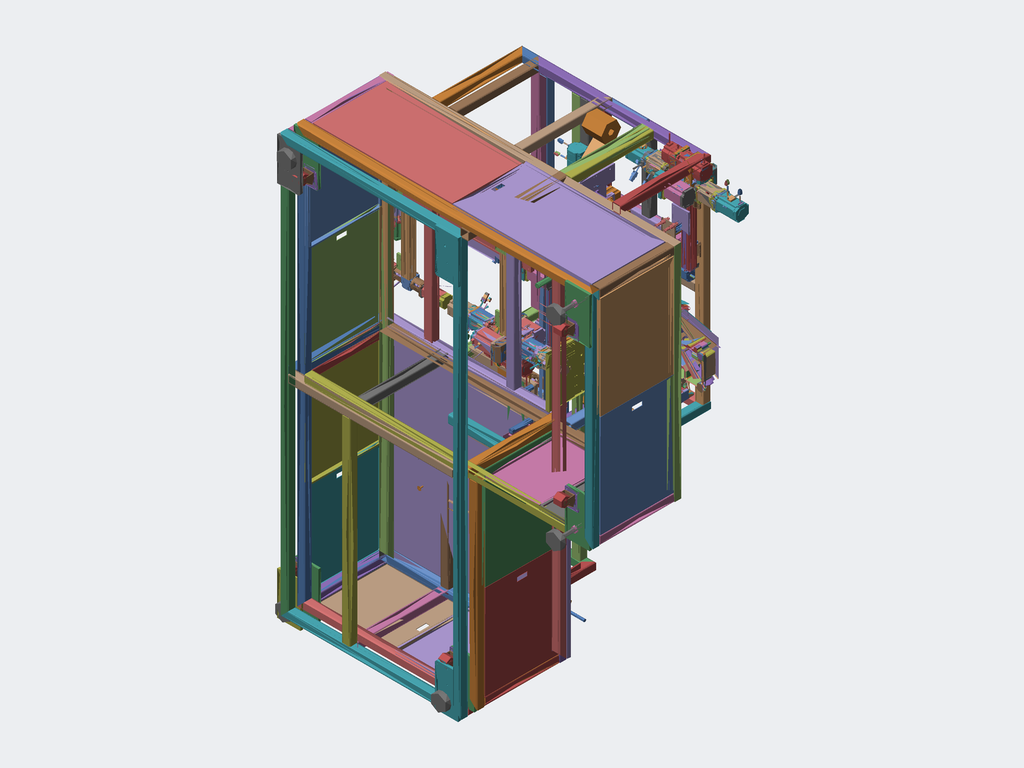Assembly | STEP file | 158 different items | 411 placed
Parts list (item | name | quantity | parent item | size | volume):
1 | - | x3 | in A14-05, A14-01 | 36 x 400 x 36 mm | 199320 mm3
2 | - | x4 | in A14-05, A14-01 | 120 x 120 x 120 mm | 1235023 mm3
3 | - | x1 | in A14-01 | 1150 x 1215 x 2550 mm | 25178560 mm3
4 | A14-004 | x1 | in A14-01 | 1200 x 20 x 1100 mm | 26268429 mm3
5 | 0303 sewing machinemodel | x1 | in A14-04 | - | -
6 | A14-006 | x8 | in A14-04 | 25 x 180 x 25 mm | 86683 mm3
7 | A14-007 | x1 | in A14-04 | 280 x 15 x 560 mm | 1039428 mm3
8 | A14-008 | x1 | in A14-04 | 290 x 20 x 750 mm | 2491365 mm3
9 | A14-005 | x2 | in 10 | 120.042 x 109.776 x 9.287 mm | 29092 mm3
10 | A14-009 | x1 | in A14-01 | - | -
11 | A14-010 | x1 | in A14-02 | 450 x 370 x 20 mm | 1407992 mm3
12 | A14-011 | x1 | in A14-02 | 450 x 370 x 20 mm | 1435092 mm3
13 | LC86HS150(shaft 14 length 32)- | x2 | in A14-02 | 86 x 86 x 182 mm | 1005876 mm3
14 | PF90-14-73-98.4-M5-20-L1 | x2 | in A14-02 | 90 x 150.5 x 90 mm | 705091 mm3
15 | A14-014 | x4 | in A14-02 | 45 x 95 x 20 mm | 53108 mm3
16 | A14-012 | x2 | in A14-02 | 60 x 310 x 60 mm | 431396 mm3
17 | A14-013 | x2 | in A14-02 | 60 x 310 x 60 mm | 430941 mm3
18 | A14-015 | x4 | in A14-02 | 40 x 14 x 39.975 mm | 13564 mm3
19 | A14-016 | x4 | in A14-02 | 280 x 16 x 16 mm | 56297 mm3
20 | A14-039 | x1 | in A14-02 | 100 x 320 x 10 mm | 307434 mm3
21 | A14-040 | x1 | in A14-02 | 38 x 320 x 10 mm | 121232 mm3
22 | - | x2 | in A14-02, A14-03 | - | -
23 | A14-018 | x1 | in A14-03 | 300 x 15 x 50 mm | 221576 mm3
24 | A14-020 | x1 | in A14-03 | 50 x 15 x 185 mm | 94203 mm3
25 | A14-021 | x1 | in A14-03 | 50 x 15 x 185 mm | 94219 mm3
26 | A14-025 | x1 | in A14-03 | 330 x 15 x 50 mm | 229412 mm3
27 | A14-019 | x1 | in A14-03 | 230 x 44 x 13 mm | 129953 mm3
28 | A14-022 | x2 | in A14-03 | 35 x 15 x 170 mm | 81962 mm3
29 | A14-028 | x1 | in A14-03 | 12 x 44 x 230 mm | 118590 mm3
30 | LSD15BK-HN-N-A-M4 | x2 | in A14-03 | 66.3 x 19.5 x 34 mm | 30804 mm3
31 | LSD15RLX170-S25-N-D | x2 | in A14-03 | 170 x 12.5 x 15 mm | 26475 mm3
32 | A14-023 | x1 | in A14-03 | 230 x 24 x 20 mm | 108684 mm3
33 | A14-024 | x1 | in A14-03 | 299 x 12 x 65 mm | 229704 mm3
34 | A14-029 | x1 | in A14-03 | - | -
35 | A14-026 | x1 | in A14-03 | 80 x 25 x 20 mm | 29104 mm3
36 | A14-027 | x1 | in A14-03 | 30 x 23 x 20 mm | 7977 mm3
37 | A14-030-1 | x1 | in A14-03 | 20 x 200 x 400 mm | 1595460 mm3
38 | A14-032 | x4 | in A14-03 | 25 x 130 x 25 mm | 62139 mm3
39 | A14-053 | x1 | in A14-03 | 204.473 x 29.929 x 260 mm | 95693 mm3
40 | - | x1 | in A14-01 | 100 x 200.5 x 1212 mm | 80600 mm3
41 | Copy of 50-2016 profile^K50A-1H20-S(formula driven)-L300-motor left- | x3 | in K50A-1H20-S(formula driven)-L300-motor left-_0 output shaft | 50 x 425 x 52.45 mm | 861534 mm3
42 | Copy of 50N support base^K50A-1H20-S(formula driven)-L300-motor left- | x6 | in K50A-1H20-S(formula driven)-L300-motor left-_0 output shaft | 82 x 32 x 80 mm | 67767 mm3
43 | Copy of K50-4 wheel slider (type B)^K50A-1H20-S(formula driven)-L300-motor left- | x3 | in K50A-1H20-S(formula driven)-L300-motor left-_0 output shaft | 140 x 34.5 x 102 mm | 434143 mm3
44 | Copy of 50-sensor^K50A-1H20-S(formula driven)-L300-motor left- | x9 | in K50A-1H20-S(formula driven)-L300-motor left-_0 output shaft | - | -
45 | Copy of K50-004 sensing plate^K50A-1H20-S(formula driven)-L300-motor left- | x3 | in K50A-1H20-S(formula driven)-L300-motor left-_0 output shaft | 20 x 33 x 15 mm | 1039 mm3
46 | Copy of K50-001A^K50A-1H20-S(formula driven)-L300-motor left- | x6 | in K50A-1H20-S(formula driven)-L300-motor left-_0 output shaft | 50 x 65 x 67.5 mm | 172642 mm3
47 | Copy of K50-right output shaft^K50A-1H20-S(formula driven)-L300-motor left- | x6 | in K50A-1H20-S(formula driven)-L300-motor left-_0 output shaft | 75.1 x 65 x 67.5 mm | 175546 mm3
48 | Copy of K50-double output shaft^K50A-1H20-S(formula driven)-L300-motor left- | x6 | in K50A-1H20-S(formula driven)-L300-motor left-_0 output shaft | 100.2 x 65 x 67.5 mm | 178596 mm3
49 | Copy of K50-left output shaft^K50A-1H20-S(formula driven)-L300-motor left- | x6 | in K50A-1H20-S(formula driven)-L300-motor left-_0 output shaft | 75.1 x 65 x 67.5 mm | 175546 mm3
50 | Copy of CZ002-400W side link 2:1(K60)^K50A-1H20-S(formula driven)-L300-motor left- | x6 | in K50A-1H20-S(formula driven)-L300-motor left-_0 output shaft | 161.001 x 70 x 175.5 mm | 580294 mm3
51 | Copy of CZ006-400W side link 3:1(K60)^K50A-1H20-S(formula driven)-L300-motor left- | x6 | in K50A-1H20-S(formula driven)-L300-motor left-_0 output shaft | 88 x 199.001 x 175.5 mm | 672015 mm3
52 | Copy of C0045-60 side link 2:1(K60)^K50A-1H20-S(formula driven)-L300-motor left- | x6 | in K50A-1H20-S(formula driven)-L300-motor left-_0 output shaft | 136.5 x 70 x 107.5 mm | 331047 mm3
53 | Copy of 400W gearbox assembly (universal motor base plus Q15)^K50A-1H20-S(formula driven)-L300-motor left- | x6 | in K50A-1H20-S(formula driven)-L300-motor left-_0 output shaft | 131.976 x 164.111 x 242.5 mm | 719537 mm3
54 | Copy of 400W motor assembly (60 motor base)^K50A-1H20-S(formula driven)-L300-motor left- | x6 | in K50A-1H20-S(formula driven)-L300-motor left-_0 output shaft | 65 x 95.5 x 200.5 mm | 502014 mm3
55 | Copy of 400W motor assembly (universal motor base)^K50A-1H20-S(formula driven)-L300-motor left- | x6 | in K50A-1H20-S(formula driven)-L300-motor left-_0 output shaft | 88.621 x 88.621 x 198.5 mm | 512392 mm3
56 | Copy of 60 motor assembly (universal motor base)^K50A-1H20-S(formula driven)-L300-motor left- | x6 | in K50A-1H20-S(formula driven)-L300-motor left-_0 output shaft | 82.65 x 82.65 x 148.5 mm | 366455 mm3
57 | Copy of 57 motor assembly (universal motor base)^K50A-1H20-S(formula driven)-L300-motor left- | x6 | in K50A-1H20-S(formula driven)-L300-motor left-_0 output shaft | 82.368 x 82.368 x 117.5 mm | 245014 mm3
58 | Copy of CZ031-57 side link 2:1(60-60N)^K50A-1H20-S(formula driven)-L300-motor left- | x6 | in K50A-1H20-S(formula driven)-L300-motor left-_0 output shaft | 60 x 146.25 x 90.3 mm | 270957 mm3
59 | Copy of CZ033-57 side link 3:1(60-60N)^K50A-1H20-S(formula driven)-L300-motor left- | x6 | in K50A-1H20-S(formula driven)-L300-motor left-_0 output shaft | 60 x 146.5 x 90.3 mm | 285335 mm3
60 | Copy of 86 motor assembly (universal motor base)^K50A-1H20-S(formula driven)-L300-motor left- | x6 | in K50A-1H20-S(formula driven)-L300-motor left-_0 output shaft | 86.045 x 86.045 x 193 mm | 941997 mm3
61 | Copy of CZ020-86 side link 2:1(K60)^K50A-1H20-S(formula driven)-L300-motor left- | x6 | in K50A-1H20-S(formula driven)-L300-motor left-_0 output shaft | 88 x 164.5 x 162 mm | 999458 mm3
62 | Copy of 90 reducer-universal motor base^K50A-1H20-S(formula driven)-L300-motor left- | x6 | in K50A-1H20-S(formula driven)-L300-motor left-_0 output shaft | 176.65 x 90 x 314 mm | 1490817 mm3
63 | Copy of 100W motor assembly (universal motor base)^K50A-1H20-S(formula driven)-L300-motor left- | x6 | in K50A-1H20-S(formula driven)-L300-motor left-_0 output shaft | 82.368 x 82.368 x 154.9 mm | 253997 mm3
64 | Copy of 750W motor assembly (universal motor base)^K50A-1H20-S(formula driven)-L300-motor left- | x6 | in K50A-1H20-S(formula driven)-L300-motor left-_0 output shaft | 82.368 x 139.887 x 214.5 mm | 943398 mm3
65 | Copy of CZ013-750W side link 2:1(K60)^K50A-1H20-S(formula driven)-L300-motor left- | x6 | in K50A-1H20-S(formula driven)-L300-motor left-_0 output shaft | 88 x 238.88 x 185 mm | 1086886 mm3
66 | Copy of hard limit assembly (right)^K50A-1H20-S(formula driven)-L300-motor left- | x3 | in K50A-1H20-S(formula driven)-L300-motor left-_0 output shaft | 24 x 15.5 x 40 mm | 6072 mm3
67 | Copy of hard limit assembly (left)^K50A-1H20-S(formula driven)-L300-motor left- | x3 | in K50A-1H20-S(formula driven)-L300-motor left-_0 output shaft | 24 x 15.5 x 40 mm | 6072 mm3
68 | A14-033 | x4 | in A14-01 | 250 x 10 x 130 mm | 324205 mm3
69 | vacuum suction cup assembly 4.5-fold bellows type standard type GXSE[GXSE-d20-20] | x8 | in A14-06 | 23.018 x 98.5 x 21.189 mm | 17845 mm3
70 | A14-034 | x3 | in A14-06, A14-13 | 10 x 100 x 120 mm | 119050 mm3
71 | A14-038 | x2 | in A14-06 | 125 x 80 x 8 mm | 15817 mm3
72 | - | x7 | in A14-06, A14-12, A14-13 | 66.5 x 47 x 20 mm | 46742 mm3
73 | A14-004-1 | x1 | in A14-01 | - | -
74 | A14-051 | x4 | in A14-10 | 25 x 207 x 25 mm | 99936 mm3
75 | A14-050 | x1 | in A14-10 | 20 x 210 x 470 mm | 1969460 mm3
76 | 311 base plate shell | x1 | in A14-11 | - | -
77 | - | x1 | in A14-11 | 100 x 58 x 40 mm | 26779 mm3
78 | 311 square head shell^2210 housing punching machine(2)_2210 housing punching machine | x1 | in A14-11 | - | -
79 | A14-052 | x1 | in A14-11 | 520 x 2 x 240 mm | 145187 mm3
80 | - | x1 | in A14-11 | 112.05 x 65 x 2.65 mm | 17494 mm3
81 | A14-062 | x1 | in A14-11 | 153 x 225 x 1.5 mm | 17798 mm3
82 | Copy of K50-right output shaft^K50A-1H20-S(formula driven)-L1200 right | x2 | in K50A-1H20-S(formula driven)-L1200 right_0 output shaft | - | -
83 | Copy of 50-sensor^K50A-1H20-S(formula driven)-L1200 right | x6 | in K50A-1H20-S(formula driven)-L1200 right_0 output shaft | 48.5 x 21.5 x 13.5 mm | 3491 mm3
84 | Copy of 50-2016 profile^K50A-1H20-S(formula driven)-L1200 right | x2 | in K50A-1H20-S(formula driven)-L1200 right_0 output shaft | 50 x 565 x 52.45 mm | 1145333 mm3
85 | Copy of 50N support base^K50A-1H20-S(formula driven)-L1200 right | x4 | in K50A-1H20-S(formula driven)-L1200 right_0 output shaft | 82 x 32 x 80 mm | 67767 mm3
86 | Copy of K50-4 wheel slider (type B)^K50A-1H20-S(formula driven)-L1200 right | x2 | in K50A-1H20-S(formula driven)-L1200 right_0 output shaft | 140 x 34.5 x 102 mm | 434143 mm3
87 | Copy of K50-left output shaft^K50A-1H20-S(formula driven)-L1200 right | x2 | in K50A-1H20-S(formula driven)-L1200 right_0 output shaft | 75.1 x 65 x 67.5 mm | 175546 mm3
88 | Copy of CZ006-400W side link 3:1(K60)^K50A-1H20-S(formula driven)-L1200 right | x2 | in K50A-1H20-S(formula driven)-L1200 right_0 output shaft | 88 x 199.001 x 175.5 mm | 672015 mm3
89 | Copy of CZ002-400W side link 2:1(K60)^K50A-1H20-S(formula driven)-L1200 right | x2 | in K50A-1H20-S(formula driven)-L1200 right_0 output shaft | 161.001 x 70 x 175.5 mm | 580294 mm3
90 | Copy of K50-001A^K50A-1H20-S(formula driven)-L1200 right | x4 | in K50A-1H20-S(formula driven)-L1200 right_0 output shaft | 50 x 65 x 67.5 mm | 172642 mm3
91 | Copy of K50-double output shaft^K50A-1H20-S(formula driven)-L1200 right | x2 | in K50A-1H20-S(formula driven)-L1200 right_0 output shaft | 100.2 x 65 x 67.5 mm | 178596 mm3
92 | Copy of K50-004 sensing plate^K50A-1H20-S(formula driven)-L1200 right | x2 | in K50A-1H20-S(formula driven)-L1200 right_0 output shaft | 20 x 33 x 15 mm | 1039 mm3
93 | Copy of 60 motor assembly (universal motor base)^K50A-1H20-S(formula driven)-L1200 right | x2 | in K50A-1H20-S(formula driven)-L1200 right_0 output shaft | 82.65 x 82.65 x 148.5 mm | 366455 mm3
94 | Copy of C0045-60 side link 2:1(K60)^K50A-1H20-S(formula driven)-L1200 right | x2 | in K50A-1H20-S(formula driven)-L1200 right_0 output shaft | 136.5 x 70 x 107.5 mm | 331047 mm3
95 | Copy of 400W gearbox assembly (universal motor base plus Q15)^K50A-1H20-S(formula driven)-L1200 right | x2 | in K50A-1H20-S(formula driven)-L1200 right_0 output shaft | 131.976 x 164.111 x 242.5 mm | 720796 mm3
96 | Copy of 400W motor assembly (universal motor base)^K50A-1H20-S(formula driven)-L1200 right | x2 | in K50A-1H20-S(formula driven)-L1200 right_0 output shaft | 88.621 x 88.621 x 198.5 mm | 512392 mm3
97 | Copy of 86 motor assembly (universal motor base)^K50A-1H20-S(formula driven)-L1200 right | x2 | in K50A-1H20-S(formula driven)-L1200 right_0 output shaft | 86.045 x 86.045 x 193 mm | 941997 mm3
98 | Copy of CZ031-57 side link 2:1(60-60N)^K50A-1H20-S(formula driven)-L1200 right | x2 | in K50A-1H20-S(formula driven)-L1200 right_0 output shaft | 60 x 146.25 x 90.3 mm | 270957 mm3
99 | Copy of 400W motor assembly (60 motor base)^K50A-1H20-S(formula driven)-L1200 right | x4 | in K50A-1H20-S(formula driven)-L1200 right_0 output shaft | - | 565676 mm3
100 | Copy of CZ033-57 side link 3:1(60-60N)^K50A-1H20-S(formula driven)-L1200 right | x2 | in K50A-1H20-S(formula driven)-L1200 right_0 output shaft | 60 x 146.5 x 90.3 mm | 285335 mm3
101 | Copy of 57 motor assembly (universal motor base)^K50A-1H20-S(formula driven)-L1200 right | x2 | in K50A-1H20-S(formula driven)-L1200 right_0 output shaft | 82.368 x 82.368 x 117.5 mm | 245014 mm3
102 | Copy of 100W motor assembly (universal motor base)^K50A-1H20-S(formula driven)-L1200 right | x2 | in K50A-1H20-S(formula driven)-L1200 right_0 output shaft | 82.368 x 82.368 x 154.9 mm | 253997 mm3
103 | Copy of 750W motor assembly (universal motor base)^K50A-1H20-S(formula driven)-L1200 right | x2 | in K50A-1H20-S(formula driven)-L1200 right_0 output shaft | 82.368 x 139.887 x 214.5 mm | 943398 mm3
104 | Copy of CZ020-86 side link 2:1(K60)^K50A-1H20-S(formula driven)-L1200 right | x2 | in K50A-1H20-S(formula driven)-L1200 right_0 output shaft | 88 x 164.5 x 162 mm | 999458 mm3
105 | Copy of CZ013-750W side link 2:1(K60)^K50A-1H20-S(formula driven)-L1200 right | x2 | in K50A-1H20-S(formula driven)-L1200 right_0 output shaft | 88 x 238.88 x 185 mm | 1086886 mm3
106 | Copy of hard limit assembly (right)^K50A-1H20-S(formula driven)-L1200 right | x1 | in K50A-1H20-S(formula driven)-L1200 right_0 output shaft | 24 x 15.5 x 40 mm | 6072 mm3
107 | Copy of 90 reducer-universal motor base^K50A-1H20-S(formula driven)-L1200 right | x2 | in K50A-1H20-S(formula driven)-L1200 right_0 output shaft | 176.65 x 90 x 314 mm | 1490817 mm3
108 | Copy of hard limit assembly (left)^K50A-1H20-S(formula driven)-L1200 right | x1 | in K50A-1H20-S(formula driven)-L1200 right_0 output shaft | 24 x 15.5 x 40 mm | 6072 mm3
109 | Copy of 50N support base^K50A-1H20-S(formula driven)-L700-motor left- | x3 | in K50A-1H20-S(formula driven)-L700-motor left-_0 output shaft | 82 x 32 x 80 mm | 67767 mm3
110 | Copy of 50-2016 profile^K50A-1H20-S(formula driven)-L700-motor left- | x1 | in K50A-1H20-S(formula driven)-L700-motor left-_0 output shaft | 50 x 815 x 52.45 mm | 1652118 mm3
111 | Copy of K50-004 sensing plate^K50A-1H20-S(formula driven)-L700-motor left- | x1 | in K50A-1H20-S(formula driven)-L700-motor left-_0 output shaft | 20 x 33 x 15 mm | 1039 mm3
112 | Copy of 50-sensor^K50A-1H20-S(formula driven)-L700-motor left- | x3 | in K50A-1H20-S(formula driven)-L700-motor left-_0 output shaft | 48.5 x 21.5 x 13.5 mm | 3491 mm3
113 | Copy of K50-001A^K50A-1H20-S(formula driven)-L700-motor left- | x2 | in K50A-1H20-S(formula driven)-L700-motor left-_0 output shaft | 50 x 65 x 67.5 mm | 172642 mm3
114 | Copy of K50-4 wheel slider (type B)^K50A-1H20-S(formula driven)-L700-motor left- | x1 | in K50A-1H20-S(formula driven)-L700-motor left-_0 output shaft | 140 x 34.5 x 102 mm | 434143 mm3
115 | Copy of CZ006-400W side link 3:1(K60)^K50A-1H20-S(formula driven)-L700-motor left- | x2 | in K50A-1H20-S(formula driven)-L700-motor left-_0 output shaft | 88 x 199.001 x 175.5 mm | 672015 mm3
116 | Copy of K50-right output shaft^K50A-1H20-S(formula driven)-L700-motor left- | x2 | in K50A-1H20-S(formula driven)-L700-motor left-_0 output shaft | 75.1 x 65 x 67.5 mm | 175722 mm3
117 | Copy of K50-double output shaft^K50A-1H20-S(formula driven)-L700-motor left- | x2 | in K50A-1H20-S(formula driven)-L700-motor left-_0 output shaft | 100.2 x 65 x 67.5 mm | 178596 mm3
118 | Copy of K50-left output shaft^K50A-1H20-S(formula driven)-L700-motor left- | x2 | in K50A-1H20-S(formula driven)-L700-motor left-_0 output shaft | 75.1 x 65 x 67.5 mm | 175546 mm3
119 | Copy of 400W motor assembly (universal motor base)^K50A-1H20-S(formula driven)-L700-motor left- | x2 | in K50A-1H20-S(formula driven)-L700-motor left-_0 output shaft | 88.621 x 88.621 x 198.5 mm | 512392 mm3
120 | Copy of 400W gearbox assembly (universal motor base plus Q15)^K50A-1H20-S(formula driven)-L700-motor left- | x2 | in K50A-1H20-S(formula driven)-L700-motor left-_0 output shaft | 131.976 x 164.111 x 242.5 mm | 719537 mm3
121 | Copy of CZ002-400W side link 2:1(K60)^K50A-1H20-S(formula driven)-L700-motor left- | x2 | in K50A-1H20-S(formula driven)-L700-motor left-_0 output shaft | 161.001 x 70 x 175.5 mm | 580294 mm3
122 | Copy of C0045-60 side link 2:1(K60)^K50A-1H20-S(formula driven)-L700-motor left- | x2 | in K50A-1H20-S(formula driven)-L700-motor left-_0 output shaft | 136.5 x 70 x 107.5 mm | 328495 mm3
123 | Copy of 400W motor assembly (60 motor base)^K50A-1H20-S(formula driven)-L700-motor left- | x2 | in K50A-1H20-S(formula driven)-L700-motor left-_0 output shaft | 65 x 95.5 x 200.5 mm | 502014 mm3
124 | Copy of 86 motor assembly (universal motor base)^K50A-1H20-S(formula driven)-L700-motor left- | x2 | in K50A-1H20-S(formula driven)-L700-motor left-_0 output shaft | 86.045 x 86.045 x 193 mm | 941997 mm3
125 | Copy of 57 motor assembly (universal motor base)^K50A-1H20-S(formula driven)-L700-motor left- | x2 | in K50A-1H20-S(formula driven)-L700-motor left-_0 output shaft | 82.368 x 82.368 x 117.5 mm | 245014 mm3
126 | Copy of CZ020-86 side link 2:1(K60)^K50A-1H20-S(formula driven)-L700-motor left- | x2 | in K50A-1H20-S(formula driven)-L700-motor left-_0 output shaft | 88 x 164.5 x 162 mm | 999458 mm3
127 | Copy of CZ033-57 side link 3:1(60-60N)^K50A-1H20-S(formula driven)-L700-motor left- | x2 | in K50A-1H20-S(formula driven)-L700-motor left-_0 output shaft | 60 x 146.5 x 90.3 mm | 285335 mm3
128 | Copy of 100W motor assembly (universal motor base)^K50A-1H20-S(formula driven)-L700-motor left- | x2 | in K50A-1H20-S(formula driven)-L700-motor left-_0 output shaft | 82.368 x 82.368 x 154.9 mm | 253997 mm3
129 | Copy of 60 motor assembly (universal motor base)^K50A-1H20-S(formula driven)-L700-motor left- | x2 | in K50A-1H20-S(formula driven)-L700-motor left-_0 output shaft | 82.65 x 82.65 x 148.5 mm | 366455 mm3
130 | Copy of CZ031-57 side link 2:1(60-60N)^K50A-1H20-S(formula driven)-L700-motor left- | x2 | in K50A-1H20-S(formula driven)-L700-motor left-_0 output shaft | 60 x 146.25 x 90.3 mm | 270957 mm3
131 | Copy of 90 reducer-universal motor base^K50A-1H20-S(formula driven)-L700-motor left- | x2 | in K50A-1H20-S(formula driven)-L700-motor left-_0 output shaft | 176.65 x 90 x 314 mm | 1490817 mm3
132 | Copy of hard limit assembly (right)^K50A-1H20-S(formula driven)-L700-motor left- | x1 | in K50A-1H20-S(formula driven)-L700-motor left-_0 output shaft | - | -
133 | Copy of 750W motor assembly (universal motor base)^K50A-1H20-S(formula driven)-L700-motor left- | x2 | in K50A-1H20-S(formula driven)-L700-motor left-_0 output shaft | 82.368 x 139.887 x 214.5 mm | 943398 mm3
134 | Copy of CZ013-750W side link 2:1(K60)^K50A-1H20-S(formula driven)-L700-motor left- | x2 | in K50A-1H20-S(formula driven)-L700-motor left-_0 output shaft | 88 x 238.88 x 185 mm | 1086886 mm3
135 | Copy of hard limit assembly (left)^K50A-1H20-S(formula driven)-L700-motor left- | x1 | in K50A-1H20-S(formula driven)-L700-motor left-_0 output shaft | 24 x 15.5 x 40 mm | 6072 mm3
136 | A14-060 | x1 | in A14-01 | 20 x 140 x 800 mm | 2235460 mm3
137 | A14-054 | x1 | in A14-12 | 430 x 10 x 480 mm | 1374000 mm3
138 | A14-057 | x1 | in A14-12 | 225 x 47 x 112.237 mm | 46754 mm3
139 | A14-056 | x1 | in A14-12 | 225 x 45 x 112.237 mm | 46079 mm3
140 | - | x2 | in A14-12 | 220 x 66.1 x 30 mm | 246050 mm3
141 | A14-055 | x1 | in A14-12 | 100 x 10 x 180 mm | 180000 mm3
142 | A14-058 | x2 | in A14-12 | 159 x 1.5 x 70 mm | 6015 mm3
143 | - | x2 | in A14-12 | 51.5 x 47 x 20 mm | 36061 mm3
144 | A14-059 | x2 | in A14-12 | 128 x 32.237 x 30 mm | 10459 mm3
145 | A14-08-1 | x1 | in A14-01 | - | -
146 | A14-061 | x1 | in A14-13 | 1.5 x 140 x 230 mm | 44100 mm3
147 | A14-08-2 | x1 | in A14-01 | - | -
148 | - | x1 | in A14-01 | 2550 x 1100 x 1800 mm | 25123488 mm3
149 | A14-066 | x5 | in A14-01 | 280 x 15 x 150 mm | 623398 mm3
150 | CGL01-D63 | x5 | in A14-01 | 82 x 96 x 111.5 mm | 244829 mm3
151 | WAM05-D100-M16-L100 | x5 | in A14-01 | 100 x 207 x 100 mm | 345017 mm3
152 | A14-Product-1 | x1 | in A14-01 | 399.758 x 100 x 500.012 mm | 1680 mm3
153 | A14-Product-2 | x1 | in A14-01 | 0.02 x 100 x 225 mm | 450 mm3
154 | - | x1 | in A14-01 | - | -
155 | Mirror Velcro | x1 | in A14-01 | 542.128 x 100 x 143.128 mm | 120000 mm3
156 | - | x1 | in Assembly 1 | 88 x 1.5 x 100 mm | 13200 mm3
157 | A14-Product-3 | x1 | in Assembly 1 | 225 x 0.2 x 100 mm | 4500 mm3
158 | - | x1 | in Assembly 1 | 55 x 1.5 x 100 mm | 8250 mm3
Placements (level | parent | child | x y z in mm | rotation matrix by rows), first 214 of 428 lines:
1 | A14-01 | A14-05 | 7.395 -242.555 146.98 | 1 0 0 0 0.995 0.1 0 -0.1 0.995
2 | A14-05 | subassembly 2 | -1394.407 492.899 1398.325 | 0 -1 0 1 0 0 0 0 1
2 | A14-05 | subassembly 2 | -1394.407 76.452 1362.677 | 0 -1 0 1 0 0 0 0 1
2 | A14-05 | subassembly 3 | -1394.407 492.899 1398.325 | 0 1 0 -0.7725 0 -0.635 -0.635 0 0.7725
1 | A14-01 | subassembly 3 | -1387.011 -30.182 1495.176 | 0 1 0 -0.7102 0 0.704 0.704 0 0.7102
1 | A14-01 | subassembly 4 | -1394.407 -687.101 2958.325 | 1 0 0 0 1 0 0 0 1
1 | A14-01 | A14-004 | -1394.407 -62.102 2283.325 | 0 0 -1 0 1 0 1 0 -0
1 | A14-01 | A14-04 | 19.784 0.0 -75.0 | 1 0 0 0 1 0 0 0 1
2 | A14-04 | 0303 sewing machinemodel | -1383.772 332.899 2064.075 | 0 -1 0 0 0 1 -1 0 0
2 | A14-04 | A14-006 | -1336.272 47.898 1955.575 | 1 0 0 0 -1 0 0 0 -1
2 | A14-04 | A14-007 | -1556.272 137.899 2070.575 | 0 0 -1 0 1 0 1 0 -0
2 | A14-04 | A14-008 | -1481.272 152.899 2070.575 | 0 0 -1 0 1 0 1 0 -0
2 | A14-04 | A14-006 | -1486.272 47.898 1955.575 | 1 0 0 0 -1 0 0 0 -1
2 | A14-04 | A14-006 | -1636.272 47.898 1955.575 | 1 0 0 0 -1 0 0 0 -1
2 | A14-04 | A14-006 | -1786.272 47.898 1955.575 | 1 0 0 0 -1 0 0 0 -1
2 | A14-04 | A14-006 | -1786.272 47.898 2185.575 | 1 0 0 0 -1 0 0 0 -1
2 | A14-04 | A14-006 | -1636.272 47.898 2185.575 | 1 0 0 0 -1 0 0 0 -1
2 | A14-04 | A14-006 | -1486.272 47.898 2185.575 | 1 0 0 0 -1 0 0 0 -1
2 | A14-04 | A14-006 | -1336.272 47.898 2185.575 | 1 0 0 0 -1 0 0 0 -1
1 | A14-01 | A14-009 | -1389.54 57.396 1881.186 | 0 -1 0 0 0 1 -1 0 -0
2 | A14-009 | A14-005 | 7.985 4.838 116.002 | 1 0 0 0 1 0 0 0 1
2 | A14-009 | A14-005 | 8.245 4.842 131.605 | 0.9994 9e-06 -0.03332 -9e-06 -1 -0.000555 -0.03332 0.000555 -0.9994
1 | A14-01 | A14-009 | -1394.407 172.899 1793.075 | 0 0 1 0 1 0 -1 0 0
1 | A14-01 | A14-02 | -1174.407 128.588 2254.397 | 0 0 -1 0 1 0 1 0 -0
2 | A14-02 | A14-010 | -8.822 14.311 370.0 | 1 0 0 0 1 0 0 0 1
2 | A14-02 | A14-011 | -8.822 14.311 70.0 | -1 0 0 0 1 0 0 0 -1
2 | A14-02 | LC86HS150(shaft 14 length 32)- | 34.178 -41.689 500.5 | 0 -1 0 -1 0 0 0 0 -1
2 | A14-02 | PF90-14-73-98.4-M5-20-L1 | -8.822 -84.689 380.0 | 1 0 0 0 0 1 0 -1 0
2 | A14-02 | A14-014 | -8.822 105.241 370.0 | 1 0 0 0 1 0 0 0 1
2 | A14-02 | A14-014 | -8.822 105.241 70.0 | -1 0 0 0 1 0 0 0 -1
2 | A14-02 | A14-012 | -8.822 77.741 375.0 | -0.8835 0 0.4684 -0.4684 0 -0.8835 0 -1 0
2 | A14-02 | A14-013 | -8.822 15.311 375.0 | 0.8247 0 -0.5656 0.5656 0 0.8247 0 -1 0
2 | A14-02 | A14-015 | 50.067 4.311 282.233 | 0.9619 0 0.2736 0.2736 0 -0.9619 0 1 -0
2 | A14-02 | A14-016 | 50.067 4.311 220.0 | 0 0 -1 0 1 0 1 0 0
2 | A14-02 | A14-016 | 50.067 -160.689 220.0 | 0 0 -1 0 1 0 1 0 0
2 | A14-02 | A14-016 | 282.289 -160.689 220.0 | 0 0 -1 0 1 0 1 0 0
2 | A14-02 | A14-016 | 282.289 4.311 220.0 | 0 0 -1 0 1 0 1 0 0
2 | A14-02 | A14-015 | 50.067 4.311 154.331 | 0.9911 0 -0.1331 -0.1331 0 -0.9911 0 1 -0
2 | A14-02 | A14-015 | 282.289 4.311 282.233 | 1 0 0 0 0 -1 0 1 -0
2 | A14-02 | A14-015 | 282.289 4.311 154.331 | 1 0 0 0 0 -1 0 1 -0
2 | A14-02 | A14-014 | 341.178 129.561 70.0 | -1 0 0 0 1 0 0 0 -1
2 | A14-02 | A14-014 | 341.178 129.561 370.0 | 1 0 0 0 1 0 0 0 1
2 | A14-02 | A14-012 | 341.178 102.061 375.0 | -0.9187 0 0.3949 -0.3949 0 -0.9187 0 -1 0
2 | A14-02 | A14-013 | 341.178 15.311 375.0 | 0.8247 0 -0.5656 0.5656 0 0.8247 0 -1 0
2 | A14-02 | PF90-14-73-98.4-M5-20-L1 | 341.178 -84.689 380.0 | 1 0 0 0 0 1 0 -1 0
2 | A14-02 | LC86HS150(shaft 14 length 32)- | 384.178 -41.689 500.5 | 0 -1 0 -1 0 0 0 0 -1
2 | A14-02 | A14-039 | 341.178 204.311 220.0 | -1 0 0 0 0 1 0 1 -0
2 | A14-02 | A14-040 | 341.178 182.061 220.0 | -1 0 0 0 0 1 0 1 -0
2 | A14-02 | subassembly 5 | 341.178 209.311 220.0 | 0 -1 0 1 0 0 0 0 1
1 | A14-01 | A14-03 | -1341.395 81.548 2180.575 | 1 0 0 0 1 0 0 0 1
2 | A14-03 | A14-018 | -53.012 33.851 520.0 | 1 0 0 0 1 0 0 0 1
2 | A14-03 | A14-020 | -203.012 118.851 520.0 | 0 -1 0 0 0 -1 1 0 0
2 | A14-03 | A14-021 | 96.988 118.851 520.0 | 0 1 0 0 0 -1 -1 0 0
2 | A14-03 | A14-025 | -53.012 211.351 520.0 | 1 0 0 0 1 0 0 0 1
2 | A14-03 | A14-019 | -53.012 63.351 538.5 | -1 0 0 0 -1 0 0 0 1
2 | A14-03 | A14-022 | 79.488 126.351 545.0 | -1 0 0 0 0 -1 0 -1 0
2 | A14-03 | A14-022 | -185.512 126.351 545.0 | -1 0 0 0 0 -1 0 -1 0
2 | A14-03 | A14-028 | -53.012 63.351 526.0 | 0 0 1 0 1 0 -1 0 -0
2 | A14-03 | LSD15BK-HN-N-A-M4 | -185.512 139.601 508.0 | 0 0 -1 1 0 0 0 -1 0
2 | A14-03 | LSD15RLX170-S25-N-D | -185.512 41.351 532.0 | 0 0 -1 1 0 0 0 -1 0
2 | A14-03 | LSD15RLX170-S25-N-D | 79.488 41.351 532.0 | 0 0 -1 1 0 0 0 -1 0
2 | A14-03 | LSD15BK-HN-N-A-M4 | 79.488 139.601 508.0 | 0 0 -1 1 0 0 0 -1 0
2 | A14-03 | A14-023 | -53.012 162.101 520.0 | 1 0 0 0 0 1 0 -1 -0
2 | A14-03 | A14-024 | -53.012 139.601 502.0 | -1 0 0 0 0 -1 0 -1 0
2 | A14-03 | A14-029 | -53.012 110.601 513.0 | 0 0 1 0 1 0 -1 0 0
2 | A14-03 | subassembly 5 | -53.012 226.351 520.0 | 0 -1 0 1 0 0 0 0 1
2 | A14-03 | A14-026 | -53.012 172.101 520.0 | 1 0 0 0 1 0 0 0 1
2 | A14-03 | A14-027 | -53.012 181.101 520.0 | 1 0 0 0 1 0 0 0 1
2 | A14-03 | A14-030-1 | -53.012 16.351 595.0 | 0 0 -1 -1 0 0 0 1 0
2 | A14-03 | A14-032 | -238.012 -58.649 680.0 | 1 0 0 0 1 0 0 0 1
2 | A14-03 | A14-032 | 131.988 -58.649 680.0 | 1 0 0 0 1 0 0 0 1
2 | A14-03 | A14-032 | 131.988 -58.649 510.0 | 1 0 0 0 1 0 0 0 1
2 | A14-03 | A14-032 | -238.012 -58.649 510.0 | -0.8428 0 -0.5383 0 1 0 0.5383 0 -0.8428
2 | A14-03 | A14-053 | -53.012 55.422 545.0 | -1 0 0 0 1 0 0 0 -1
1 | A14-01 | subassembly 6 | -1394.407 174.149 3024.964 | 1 0 0 0 1 0 0 0 1
1 | A14-01 | K50A-1H20-S(formula driven)-L300-motor left-_0 output shaft | -1394.407 417.899 3242.575 | 1 0 0 0 -1 0 0 0 -1
2 | K50A-1H20-S(formula driven)-L300-motor left-_0 output shaft | Copy of 50-2016 profile^K50A-1H20-S(formula driven)-L300-motor left- | -0.0 -0.0 -0.0 | 1 0 0 0 0 -1 0 1 0
2 | K50A-1H20-S(formula driven)-L300-motor left-_0 output shaft | Copy of 50N support base^K50A-1H20-S(formula driven)-L300-motor left- | -0.0 -10.0 335.0 | 1 0 0 0 1 0 0 0 1
2 | K50A-1H20-S(formula driven)-L300-motor left-_0 output shaft | Copy of K50-4 wheel slider (type B)^K50A-1H20-S(formula driven)-L300-motor left- | 142.0 50.55 347.856 | 0 0 -1 0 1 0 1 0 0
2 | K50A-1H20-S(formula driven)-L300-motor left-_0 output shaft | Copy of 50-sensor^K50A-1H20-S(formula driven)-L300-motor left- | 24.949 47.3 400.945 | 0 1 0 0 0 -1 -1 0 0
2 | K50A-1H20-S(formula driven)-L300-motor left-_0 output shaft | Copy of K50-004 sensing plate^K50A-1H20-S(formula driven)-L300-motor left- | 52.2 30.2 396.016 | 0 0 1 0 1 0 -1 0 -0
2 | K50A-1H20-S(formula driven)-L300-motor left-_0 output shaft | Copy of 50-sensor^K50A-1H20-S(formula driven)-L300-motor left- | 24.949 47.3 130.144 | 0 1 0 0 0 -1 -1 0 0
2 | K50A-1H20-S(formula driven)-L300-motor left-_0 output shaft | Copy of 50-sensor^K50A-1H20-S(formula driven)-L300-motor left- | 24.949 47.3 181.144 | 0 1 0 0 0 -1 -1 0 0
2 | K50A-1H20-S(formula driven)-L300-motor left-_0 output shaft | Copy of K50-001A^K50A-1H20-S(formula driven)-L300-motor left- | -1.386 27.562 -25.0 | 1 0 0 0 1 0 0 0 1
2 | K50A-1H20-S(formula driven)-L300-motor left-_0 output shaft | Copy of K50-001A^K50A-1H20-S(formula driven)-L300-motor left- | 1.386 27.562 450.0 | -1 0 0 0 1 0 0 0 -1
2 | K50A-1H20-S(formula driven)-L300-motor left-_0 output shaft | Copy of K50-right output shaft^K50A-1H20-S(formula driven)-L300-motor left- | 1.386 27.562 450.0 | -1 0 0 0 1 0 0 0 -1
2 | K50A-1H20-S(formula driven)-L300-motor left-_0 output shaft | Copy of K50-right output shaft^K50A-1H20-S(formula driven)-L300-motor left- | -1.386 27.562 -25.0 | 1 0 0 0 1 0 0 0 1
2 | K50A-1H20-S(formula driven)-L300-motor left-_0 output shaft | Copy of K50-double output shaft^K50A-1H20-S(formula driven)-L300-motor left- | -1.386 27.562 -25.0 | 1 0 0 0 1 0 0 0 1
2 | K50A-1H20-S(formula driven)-L300-motor left-_0 output shaft | Copy of K50-double output shaft^K50A-1H20-S(formula driven)-L300-motor left- | 1.386 27.562 450.0 | -1 0 0 0 1 0 0 0 -1
2 | K50A-1H20-S(formula driven)-L300-motor left-_0 output shaft | Copy of K50-left output shaft^K50A-1H20-S(formula driven)-L300-motor left- | -1.386 27.562 -25.0 | 1 0 0 0 1 0 0 0 1
2 | K50A-1H20-S(formula driven)-L300-motor left-_0 output shaft | Copy of K50-left output shaft^K50A-1H20-S(formula driven)-L300-motor left- | 1.386 27.562 450.0 | -1 0 0 0 1 0 0 0 -1
2 | K50A-1H20-S(formula driven)-L300-motor left-_0 output shaft | Copy of 50N support base^K50A-1H20-S(formula driven)-L300-motor left- | -0.0 -10.0 79.0 | 1 0 0 0 1 0 0 0 1
2 | K50A-1H20-S(formula driven)-L300-motor left-_0 output shaft | Copy of CZ002-400W side link 2:1(K60)^K50A-1H20-S(formula driven)-L300-motor left- | -137.949 50.063 -41.164 | 0 0 1 -1 0 0 0 -1 0
2 | K50A-1H20-S(formula driven)-L300-motor left-_0 output shaft | Copy of CZ006-400W side link 3:1(K60)^K50A-1H20-S(formula driven)-L300-motor left- | -139.254 -53.524 5.303 | 0 0 1 0 -1 0 1 0 -0
2 | K50A-1H20-S(formula driven)-L300-motor left-_0 output shaft | Copy of CZ006-400W side link 3:1(K60)^K50A-1H20-S(formula driven)-L300-motor left- | 139.254 70.303 -118.524 | 0 0 -1 1 0 0 0 -1 -0
2 | K50A-1H20-S(formula driven)-L300-motor left-_0 output shaft | Copy of CZ002-400W side link 2:1(K60)^K50A-1H20-S(formula driven)-L300-motor left- | 137.949 46.164 -45.063 | 0 0 -1 0 1 0 1 0 0
2 | K50A-1H20-S(formula driven)-L300-motor left-_0 output shaft | Copy of C0045-60 side link 2:1(K60)^K50A-1H20-S(formula driven)-L300-motor left- | -137.949 50.063 -41.164 | 0 0 1 -1 0 0 0 -1 0
2 | K50A-1H20-S(formula driven)-L300-motor left-_0 output shaft | Copy of C0045-60 side link 2:1(K60)^K50A-1H20-S(formula driven)-L300-motor left- | 137.949 46.164 -45.063 | 0 0 -1 0 1 0 1 0 -0
2 | K50A-1H20-S(formula driven)-L300-motor left-_0 output shaft | Copy of 400W gearbox assembly (universal motor base plus Q15)^K50A-1H20-S(formula driven)-L300-motor left- | 28.0 35.0 -30.0 | 0 0 1 0 1 0 -1 0 0
2 | K50A-1H20-S(formula driven)-L300-motor left-_0 output shaft | Copy of 400W motor assembly (60 motor base)^K50A-1H20-S(formula driven)-L300-motor left- | 58.836 40.482 14.041 | 0 0 -1 0 -1 0 -1 0 0
2 | K50A-1H20-S(formula driven)-L300-motor left-_0 output shaft | Copy of 400W motor assembly (universal motor base)^K50A-1H20-S(formula driven)-L300-motor left- | -25.868 28.042 -17.555 | 0 0 1 0 1 0 -1 0 0
2 | K50A-1H20-S(formula driven)-L300-motor left-_0 output shaft | Copy of 400W gearbox assembly (universal motor base plus Q15)^K50A-1H20-S(formula driven)-L300-motor left- | -28.0 35.0 -30.0 | 0 0 -1 0 -1 0 -1 0 -0
2 | K50A-1H20-S(formula driven)-L300-motor left-_0 output shaft | Copy of 400W motor assembly (universal motor base)^K50A-1H20-S(formula driven)-L300-motor left- | 25.868 41.958 -17.555 | 0 0 -1 0 -1 0 -1 0 -0
2 | K50A-1H20-S(formula driven)-L300-motor left-_0 output shaft | Copy of 400W motor assembly (60 motor base)^K50A-1H20-S(formula driven)-L300-motor left- | -58.836 29.518 14.041 | 0 0 1 0 1 0 -1 0 -0
2 | K50A-1H20-S(formula driven)-L300-motor left-_0 output shaft | Copy of 60 motor assembly (universal motor base)^K50A-1H20-S(formula driven)-L300-motor left- | 25.868 42.444 -32.04 | 0 0 -1 0 -1 0 -1 0 -0
2 | K50A-1H20-S(formula driven)-L300-motor left-_0 output shaft | Copy of 60 motor assembly (universal motor base)^K50A-1H20-S(formula driven)-L300-motor left- | -25.868 27.556 -32.04 | 0 0 1 0 1 0 -1 0 0
2 | K50A-1H20-S(formula driven)-L300-motor left-_0 output shaft | Copy of 57 motor assembly (universal motor base)^K50A-1H20-S(formula driven)-L300-motor left- | -25.867 39.661 -53.676 | 0 0 1 0 1 0 -1 0 0
2 | K50A-1H20-S(formula driven)-L300-motor left-_0 output shaft | Copy of CZ031-57 side link 2:1(60-60N)^K50A-1H20-S(formula driven)-L300-motor left- | -107.0 78.623 -31.684 | 0 0 1 0 1 0 -1 0 0
2 | K50A-1H20-S(formula driven)-L300-motor left-_0 output shaft | Copy of CZ033-57 side link 3:1(60-60N)^K50A-1H20-S(formula driven)-L300-motor left- | -107.0 78.623 -31.684 | 0 0 1 0 1 0 -1 0 -0
2 | K50A-1H20-S(formula driven)-L300-motor left-_0 output shaft | Copy of CZ033-57 side link 3:1(60-60N)^K50A-1H20-S(formula driven)-L300-motor left- | 107.0 36.684 -73.623 | 0 0 -1 1 0 0 0 -1 -0
2 | K50A-1H20-S(formula driven)-L300-motor left-_0 output shaft | Copy of CZ031-57 side link 2:1(60-60N)^K50A-1H20-S(formula driven)-L300-motor left- | 107.0 36.684 -73.623 | 0 0 -1 1 0 0 0 -1 -0
2 | K50A-1H20-S(formula driven)-L300-motor left-_0 output shaft | Copy of 57 motor assembly (universal motor base)^K50A-1H20-S(formula driven)-L300-motor left- | 25.867 30.339 -53.676 | 0 0 -1 0 -1 0 -1 0 -0
2 | K50A-1H20-S(formula driven)-L300-motor left-_0 output shaft | Copy of 86 motor assembly (universal motor base)^K50A-1H20-S(formula driven)-L300-motor left- | -25.868 26.685 -28.19 | 0 0 1 0 1 0 -1 0 0
2 | K50A-1H20-S(formula driven)-L300-motor left-_0 output shaft | Copy of 86 motor assembly (universal motor base)^K50A-1H20-S(formula driven)-L300-motor left- | 25.868 43.315 -28.19 | 0 0 -1 0 -1 0 -1 0 -0
2 | K50A-1H20-S(formula driven)-L300-motor left-_0 output shaft | Copy of CZ020-86 side link 2:1(K60)^K50A-1H20-S(formula driven)-L300-motor left- | -131.645 -38.755 -4.508 | 0 0 1 0 -1 0 1 0 0
2 | K50A-1H20-S(formula driven)-L300-motor left-_0 output shaft | Copy of CZ020-86 side link 2:1(K60)^K50A-1H20-S(formula driven)-L300-motor left- | 131.645 108.755 -4.508 | 0 0 -1 0 1 0 1 0 0
2 | K50A-1H20-S(formula driven)-L300-motor left-_0 output shaft | Copy of 90 reducer-universal motor base^K50A-1H20-S(formula driven)-L300-motor left- | 4.902 63.56 -46.01 | 0 0 1 0 1 0 -1 0 0
2 | K50A-1H20-S(formula driven)-L300-motor left-_0 output shaft | Copy of 90 reducer-universal motor base^K50A-1H20-S(formula driven)-L300-motor left- | -4.902 6.44 -46.01 | 0 0 -1 0 -1 0 -1 0 -0
2 | K50A-1H20-S(formula driven)-L300-motor left-_0 output shaft | Copy of 100W motor assembly (universal motor base)^K50A-1H20-S(formula driven)-L300-motor left- | -25.868 30.418 -8.844 | 0 0 1 0 1 0 -1 0 0
2 | K50A-1H20-S(formula driven)-L300-motor left-_0 output shaft | Copy of 100W motor assembly (universal motor base)^K50A-1H20-S(formula driven)-L300-motor left- | 25.868 39.582 -8.844 | 0 0 -1 0 -1 0 -1 0 -0
2 | K50A-1H20-S(formula driven)-L300-motor left-_0 output shaft | Copy of 750W motor assembly (universal motor base)^K50A-1H20-S(formula driven)-L300-motor left- | -25.868 36.188 -29.887 | 0 0 1 0 1 0 -1 0 0
2 | K50A-1H20-S(formula driven)-L300-motor left-_0 output shaft | Copy of CZ013-750W side link 2:1(K60)^K50A-1H20-S(formula driven)-L300-motor left- | -83.709 -0.3027 -12.512 | 0 0 1 -1 0 0 0 -1 0
2 | K50A-1H20-S(formula driven)-L300-motor left-_0 output shaft | Copy of CZ013-750W side link 2:1(K60)^K50A-1H20-S(formula driven)-L300-motor left- | 83.709 70.303 -12.512 | 0 0 -1 1 0 0 0 -1 -0
2 | K50A-1H20-S(formula driven)-L300-motor left-_0 output shaft | Copy of 750W motor assembly (universal motor base)^K50A-1H20-S(formula driven)-L300-motor left- | 25.868 33.812 -29.887 | 0 0 -1 0 -1 0 -1 0 -0
2 | K50A-1H20-S(formula driven)-L300-motor left-_0 output shaft | Copy of hard limit assembly (right)^K50A-1H20-S(formula driven)-L300-motor left- | -31.412 -15.95 284.418 | 0 -1 0 0 0 1 -1 0 0
2 | K50A-1H20-S(formula driven)-L300-motor left-_0 output shaft | Copy of hard limit assembly (left)^K50A-1H20-S(formula driven)-L300-motor left- | 31.913 -15.95 288.592 | 0 1 0 0 0 1 1 0 -0
1 | A14-01 | A14-033 | -1394.407 432.899 3163.575 | 1 0 0 0 1 0 0 0 1
1 | A14-01 | A14-033 | -1394.407 432.899 2907.575 | 1 0 0 0 1 0 0 0 1
1 | A14-01 | A14-06 | -1383.439 353.157 2781.559 | 0 -1 0 1 0 0 0 0 1
2 | A14-06 | vacuum suction cup assembly 4.5-fold bellows type standard type GXSE[GXSE-d20-20] | -68.259 -14.796 32.5 | 0 1 0 0.7043 0 -0.7099 -0.7099 0 -0.7043
2 | A14-06 | vacuum suction cup assembly 4.5-fold bellows type standard type GXSE[GXSE-d20-20] | -68.259 36.731 32.5 | 0 1 0 0.7043 0 -0.7099 -0.7099 0 -0.7043
2 | A14-06 | vacuum suction cup assembly 4.5-fold bellows type standard type GXSE[GXSE-d20-20] | -68.259 36.731 133.5 | 0 1 0 0.7043 0 -0.7099 -0.7099 0 -0.7043
2 | A14-06 | A14-034 | -7.259 10.968 120.0 | 1 0 0 0 1 0 0 0 1
2 | A14-06 | A14-038 | -80.259 10.968 83.0 | 0 0 1 0 1 0 -1 0 -0
2 | A14-06 | subassembly 7 | -67.259 10.968 90.5 | 1 0 0 0 0 1 0 -1 -0
2 | A14-06 | vacuum suction cup assembly 4.5-fold bellows type standard type GXSE[GXSE-d20-20] | -68.259 -14.796 133.5 | 0 1 0 0.7043 0 -0.7099 -0.7099 0 -0.7043
1 | A14-01 | A14-004-1 | -1044.407 -62.102 3558.325 | 0 0 1 0 1 0 -1 0 0
1 | A14-01 | A14-10 | -429.012 196.381 3619.4 | 0 0 -1 -1 0 0 0 1 0
2 | A14-10 | A14-051 | 134.983 97.725 620.0 | 0 1 0 -0.3621 0 -0.9321 -0.9321 0 0.3621
2 | A14-10 | A14-050 | 21.483 7.725 400.0 | 1 0 0 0 1 0 0 0 1
2 | A14-10 | A14-051 | 134.983 97.725 180.0 | 0 1 0 -0.3621 0 -0.9321 -0.9321 0 0.3621
2 | A14-10 | A14-051 | 134.983 -82.275 180.0 | 0 1 0 -0.3621 0 -0.9321 -0.9321 0 0.3621
2 | A14-10 | A14-051 | 134.983 -82.275 620.0 | 0 1 0 -0.3621 0 -0.9321 -0.9321 0 0.3621
1 | A14-01 | A14-11 | 553.461 105.81 -561.939 | 1 0 0 0 1 0 0 0 1
2 | A14-11 | 311 base plate shell | -1229.036 41.689 4033.864 | 0 -1 0 0 0 -1 1 0 -0
2 | A14-11 | subassembly 8 | -1152.34 87.848 4044.166 | 0 0 -1 0 1 0 1 0 -0
2 | A14-11 | 311 square head shell^2210 housing punching machine(2)_2210 housing punching machine | -706.252 265.288 4033.814 | -1 0 0 0 0 -1 0 -1 -0
2 | A14-11 | A14-052 | -1247.472 78.088 4034.064 | 0 0 -1 0 1 0 1 0 -0
2 | A14-11 | subassembly 9 | -1180.472 76.439 4001.364 | -1 0 0 0 0 1 0 1 0
2 | A14-11 | A14-062 | -1233.254 87.848 4141.666 | 1 0 0 0 0 1 0 -1 0
1 | A14-01 | K50A-1H20-S(formula driven)-L1200 right_0 output shaft | -1263.407 -32.102 3165.575 | 1 0 0 0 1 0 0 0 1
2 | K50A-1H20-S(formula driven)-L1200 right_0 output shaft | Copy of K50-right output shaft^K50A-1H20-S(formula driven)-L1200 right | -1.386 27.562 115.0 | 1 0 0 0 1 0 0 0 1
2 | K50A-1H20-S(formula driven)-L1200 right_0 output shaft | Copy of 50-sensor^K50A-1H20-S(formula driven)-L1200 right | 24.949 47.3 540.944 | 0 1 0 0 0 -1 -1 0 0
2 | K50A-1H20-S(formula driven)-L1200 right_0 output shaft | Copy of 50-2016 profile^K50A-1H20-S(formula driven)-L1200 right | -0.0 -0.0 -0.0 | 1 0 0 0 0 -1 0 1 0
2 | K50A-1H20-S(formula driven)-L1200 right_0 output shaft | Copy of 50N support base^K50A-1H20-S(formula driven)-L1200 right | 0.0 -10.0 475.0 | 1 0 0 0 1 0 0 0 1
2 | K50A-1H20-S(formula driven)-L1200 right_0 output shaft | Copy of K50-4 wheel slider (type B)^K50A-1H20-S(formula driven)-L1200 right | 142.0 50.55 421.535 | 0 0 -1 0 1 0 1 0 0
2 | K50A-1H20-S(formula driven)-L1200 right_0 output shaft | Copy of K50-left output shaft^K50A-1H20-S(formula driven)-L1200 right | 1.386 27.562 450.0 | -1 0 0 0 1 0 0 0 -1
2 | K50A-1H20-S(formula driven)-L1200 right_0 output shaft | Copy of CZ006-400W side link 3:1(K60)^K50A-1H20-S(formula driven)-L1200 right | -139.254 -53.524 5.303 | 0 0 1 0 -1 0 1 0 -0
2 | K50A-1H20-S(formula driven)-L1200 right_0 output shaft | Copy of CZ002-400W side link 2:1(K60)^K50A-1H20-S(formula driven)-L1200 right | 137.949 46.164 -45.063 | 0 0 -1 0 1 0 1 0 0
2 | K50A-1H20-S(formula driven)-L1200 right_0 output shaft | Copy of 50-sensor^K50A-1H20-S(formula driven)-L1200 right | 24.949 47.3 181.144 | 0 1 0 0 0 -1 -1 0 0
2 | K50A-1H20-S(formula driven)-L1200 right_0 output shaft | Copy of K50-001A^K50A-1H20-S(formula driven)-L1200 right | -1.386 27.562 115.0 | 1 0 0 0 1 0 0 0 1
2 | K50A-1H20-S(formula driven)-L1200 right_0 output shaft | Copy of K50-double output shaft^K50A-1H20-S(formula driven)-L1200 right | -1.386 27.562 115.0 | 1 0 0 0 1 0 0 0 1
2 | K50A-1H20-S(formula driven)-L1200 right_0 output shaft | Copy of 50-sensor^K50A-1H20-S(formula driven)-L1200 right | 24.949 47.3 130.144 | 0 1 0 0 0 -1 -1 0 0
2 | K50A-1H20-S(formula driven)-L1200 right_0 output shaft | Copy of K50-right output shaft^K50A-1H20-S(formula driven)-L1200 right | 1.386 27.562 450.0 | -1 0 0 0 1 0 0 0 -1
2 | K50A-1H20-S(formula driven)-L1200 right_0 output shaft | Copy of K50-001A^K50A-1H20-S(formula driven)-L1200 right | 1.386 27.562 450.0 | -1 0 0 0 1 0 0 0 -1
2 | K50A-1H20-S(formula driven)-L1200 right_0 output shaft | Copy of K50-004 sensing plate^K50A-1H20-S(formula driven)-L1200 right | 52.2 30.2 469.695 | 0 0 1 0 1 0 -1 0 -0
2 | K50A-1H20-S(formula driven)-L1200 right_0 output shaft | Copy of K50-double output shaft^K50A-1H20-S(formula driven)-L1200 right | 1.386 27.562 450.0 | -1 0 0 0 1 0 0 0 -1
2 | K50A-1H20-S(formula driven)-L1200 right_0 output shaft | Copy of K50-left output shaft^K50A-1H20-S(formula driven)-L1200 right | -1.386 27.562 115.0 | 1 0 0 0 1 0 0 0 1
2 | K50A-1H20-S(formula driven)-L1200 right_0 output shaft | Copy of CZ002-400W side link 2:1(K60)^K50A-1H20-S(formula driven)-L1200 right | -137.949 50.063 -41.164 | 0 0 1 -1 0 0 0 -1 0
2 | K50A-1H20-S(formula driven)-L1200 right_0 output shaft | Copy of CZ006-400W side link 3:1(K60)^K50A-1H20-S(formula driven)-L1200 right | 139.254 70.303 -118.524 | 0 0 -1 1 0 0 0 -1 -0
2 | K50A-1H20-S(formula driven)-L1200 right_0 output shaft | Copy of 60 motor assembly (universal motor base)^K50A-1H20-S(formula driven)-L1200 right | 25.868 42.444 -32.04 | 0 0 -1 0 -1 0 -1 0 -0
2 | K50A-1H20-S(formula driven)-L1200 right_0 output shaft | Copy of C0045-60 side link 2:1(K60)^K50A-1H20-S(formula driven)-L1200 right | -137.949 50.063 -41.164 | 0 0 1 -1 0 0 0 -1 0
2 | K50A-1H20-S(formula driven)-L1200 right_0 output shaft | Copy of 400W gearbox assembly (universal motor base plus Q15)^K50A-1H20-S(formula driven)-L1200 right | 28.0 35.0 -30.0 | 0 0 1 0 1 0 -1 0 0
2 | K50A-1H20-S(formula driven)-L1200 right_0 output shaft | Copy of 400W motor assembly (universal motor base)^K50A-1H20-S(formula driven)-L1200 right | -25.868 28.042 -17.555 | 0 0 1 0 1 0 -1 0 0
2 | K50A-1H20-S(formula driven)-L1200 right_0 output shaft | Copy of 400W gearbox assembly (universal motor base plus Q15)^K50A-1H20-S(formula driven)-L1200 right | -28.0 35.0 -30.0 | 0 0 -1 0 -1 0 -1 0 -0
2 | K50A-1H20-S(formula driven)-L1200 right_0 output shaft | Copy of 86 motor assembly (universal motor base)^K50A-1H20-S(formula driven)-L1200 right | -25.868 26.685 -28.19 | 0 0 1 0 1 0 -1 0 0
2 | K50A-1H20-S(formula driven)-L1200 right_0 output shaft | Copy of CZ031-57 side link 2:1(60-60N)^K50A-1H20-S(formula driven)-L1200 right | -107.0 78.623 -31.684 | 0 0 1 0 1 0 -1 0 0
2 | K50A-1H20-S(formula driven)-L1200 right_0 output shaft | Copy of 400W motor assembly (universal motor base)^K50A-1H20-S(formula driven)-L1200 right | 25.868 41.958 -17.555 | 0 0 -1 0 -1 0 -1 0 -0
2 | K50A-1H20-S(formula driven)-L1200 right_0 output shaft | Copy of 400W motor assembly (60 motor base)^K50A-1H20-S(formula driven)-L1200 right | 58.836 40.482 14.041 | 0 0 -1 0 -1 0 -1 0 0
2 | K50A-1H20-S(formula driven)-L1200 right_0 output shaft | Copy of 400W motor assembly (60 motor base)^K50A-1H20-S(formula driven)-L1200 right | -58.836 29.518 14.041 | 0 0 1 0 1 0 -1 0 -0
2 | K50A-1H20-S(formula driven)-L1200 right_0 output shaft | Copy of C0045-60 side link 2:1(K60)^K50A-1H20-S(formula driven)-L1200 right | 137.949 46.164 -45.063 | 0 0 -1 0 1 0 1 0 -0
2 | K50A-1H20-S(formula driven)-L1200 right_0 output shaft | Copy of CZ033-57 side link 3:1(60-60N)^K50A-1H20-S(formula driven)-L1200 right | -107.0 78.623 -31.684 | 0 0 1 0 1 0 -1 0 -0
2 | K50A-1H20-S(formula driven)-L1200 right_0 output shaft | Copy of 57 motor assembly (universal motor base)^K50A-1H20-S(formula driven)-L1200 right | -25.867 39.661 -53.676 | 0 0 1 0 1 0 -1 0 0
2 | K50A-1H20-S(formula driven)-L1200 right_0 output shaft | Copy of 60 motor assembly (universal motor base)^K50A-1H20-S(formula driven)-L1200 right | -25.868 27.556 -32.04 | 0 0 1 0 1 0 -1 0 0
2 | K50A-1H20-S(formula driven)-L1200 right_0 output shaft | Copy of CZ033-57 side link 3:1(60-60N)^K50A-1H20-S(formula driven)-L1200 right | 107.0 36.684 -73.623 | 0 0 -1 1 0 0 0 -1 -0
2 | K50A-1H20-S(formula driven)-L1200 right_0 output shaft | Copy of CZ031-57 side link 2:1(60-60N)^K50A-1H20-S(formula driven)-L1200 right | 107.0 36.684 -73.623 | 0 0 -1 1 0 0 0 -1 -0
2 | K50A-1H20-S(formula driven)-L1200 right_0 output shaft | Copy of 57 motor assembly (universal motor base)^K50A-1H20-S(formula driven)-L1200 right | 25.867 30.339 -53.676 | 0 0 -1 0 -1 0 -1 0 -0
2 | K50A-1H20-S(formula driven)-L1200 right_0 output shaft | Copy of 86 motor assembly (universal motor base)^K50A-1H20-S(formula driven)-L1200 right | 25.868 43.315 -28.19 | 0 0 -1 0 -1 0 -1 0 -0
2 | K50A-1H20-S(formula driven)-L1200 right_0 output shaft | Copy of 50N support base^K50A-1H20-S(formula driven)-L1200 right | 0.0 -10.0 79.0 | 1 0 0 0 1 0 0 0 1
2 | K50A-1H20-S(formula driven)-L1200 right_0 output shaft | Copy of 50N support base^K50A-1H20-S(formula driven)-L1200 right | -600.0 -10.0 79.0 | 1 0 0 0 1 0 0 0 1
2 | K50A-1H20-S(formula driven)-L1200 right_0 output shaft | Copy of K50-004 sensing plate^K50A-1H20-S(formula driven)-L1200 right | -547.8 30.2 469.695 | 0 0 1 0 1 0 -1 0 -0
2 | K50A-1H20-S(formula driven)-L1200 right_0 output shaft | Copy of K50-001A^K50A-1H20-S(formula driven)-L1200 right | -601.386 27.562 115.0 | 1 0 0 0 1 0 0 0 1
2 | K50A-1H20-S(formula driven)-L1200 right_0 output shaft | Copy of 50-sensor^K50A-1H20-S(formula driven)-L1200 right | -575.051 47.3 130.144 | 0 1 0 0 0 -1 -1 0 0
2 | K50A-1H20-S(formula driven)-L1200 right_0 output shaft | Copy of 50-2016 profile^K50A-1H20-S(formula driven)-L1200 right | -600.0 0.0 -0.0 | 1 0 0 0 0 -1 0 1 0
2 | K50A-1H20-S(formula driven)-L1200 right_0 output shaft | Copy of 50-sensor^K50A-1H20-S(formula driven)-L1200 right | -575.051 47.3 540.944 | 0 1 0 0 0 -1 -1 0 0
2 | K50A-1H20-S(formula driven)-L1200 right_0 output shaft | Copy of 50N support base^K50A-1H20-S(formula driven)-L1200 right | -600.0 -10.0 475.0 | 1 0 0 0 1 0 0 0 1
2 | K50A-1H20-S(formula driven)-L1200 right_0 output shaft | Copy of K50-4 wheel slider (type B)^K50A-1H20-S(formula driven)-L1200 right | -458.0 50.55 421.535 | 0 0 -1 0 1 0 1 0 0
2 | K50A-1H20-S(formula driven)-L1200 right_0 output shaft | Copy of 400W motor assembly (60 motor base)^K50A-1H20-S(formula driven)-L1200 right | -541.164 40.482 14.041 | 0 0 -1 0 -1 0 -1 0 0
2 | K50A-1H20-S(formula driven)-L1200 right_0 output shaft | Copy of 50-sensor^K50A-1H20-S(formula driven)-L1200 right | -575.051 47.3 181.144 | 0 1 0 0 0 -1 -1 0 0
2 | K50A-1H20-S(formula driven)-L1200 right_0 output shaft | Copy of K50-001A^K50A-1H20-S(formula driven)-L1200 right | -598.614 27.562 450.0 | -1 0 0 0 1 0 0 0 -1
2 | K50A-1H20-S(formula driven)-L1200 right_0 output shaft | Copy of 400W motor assembly (60 motor base)^K50A-1H20-S(formula driven)-L1200 right | -658.836 29.518 14.041 | 0 0 1 0 1 0 -1 0 -0
2 | K50A-1H20-S(formula driven)-L1200 right_0 output shaft | Copy of 100W motor assembly (universal motor base)^K50A-1H20-S(formula driven)-L1200 right | -25.868 30.418 -8.844 | 0 0 1 0 1 0 -1 0 0
2 | K50A-1H20-S(formula driven)-L1200 right_0 output shaft | Copy of 750W motor assembly (universal motor base)^K50A-1H20-S(formula driven)-L1200 right | 25.868 33.812 -29.887 | 0 0 -1 0 -1 0 -1 0 -0
2 | K50A-1H20-S(formula driven)-L1200 right_0 output shaft | Copy of CZ020-86 side link 2:1(K60)^K50A-1H20-S(formula driven)-L1200 right | 131.645 108.755 -4.508 | 0 0 -1 0 1 0 1 0 0
2 | K50A-1H20-S(formula driven)-L1200 right_0 output shaft | Copy of CZ013-750W side link 2:1(K60)^K50A-1H20-S(formula driven)-L1200 right | 83.709 70.303 -12.512 | 0 0 -1 1 0 0 0 -1 -0
2 | K50A-1H20-S(formula driven)-L1200 right_0 output shaft | Copy of CZ013-750W side link 2:1(K60)^K50A-1H20-S(formula driven)-L1200 right | -83.709 -0.3027 -12.512 | 0 0 1 -1 0 0 0 -1 0
2 | K50A-1H20-S(formula driven)-L1200 right_0 output shaft | Copy of hard limit assembly (right)^K50A-1H20-S(formula driven)-L1200 right | -31.412 -15.95 14.722 | 0 -1 0 0 0 1 -1 0 0
2 | K50A-1H20-S(formula driven)-L1200 right_0 output shaft | Copy of 90 reducer-universal motor base^K50A-1H20-S(formula driven)-L1200 right | -4.902 6.44 -46.01 | 0 0 -1 0 -1 0 -1 0 -0
2 | K50A-1H20-S(formula driven)-L1200 right_0 output shaft | Copy of 90 reducer-universal motor base^K50A-1H20-S(formula driven)-L1200 right | 4.902 63.56 -46.01 | 0 0 1 0 1 0 -1 0 0
2 | K50A-1H20-S(formula driven)-L1200 right_0 output shaft | Copy of CZ020-86 side link 2:1(K60)^K50A-1H20-S(formula driven)-L1200 right | -131.645 -38.755 -4.508 | 0 0 1 0 -1 0 1 0 0
2 | K50A-1H20-S(formula driven)-L1200 right_0 output shaft | Copy of 100W motor assembly (universal motor base)^K50A-1H20-S(formula driven)-L1200 right | 25.868 39.582 -8.844 | 0 0 -1 0 -1 0 -1 0 -0
2 | K50A-1H20-S(formula driven)-L1200 right_0 output shaft | Copy of 750W motor assembly (universal motor base)^K50A-1H20-S(formula driven)-L1200 right | -25.868 36.188 -29.887 | 0 0 1 0 1 0 -1 0 0
2 | K50A-1H20-S(formula driven)-L1200 right_0 output shaft | Copy of hard limit assembly (left)^K50A-1H20-S(formula driven)-L1200 right | 31.913 -15.95 20.751 | 0 1 0 0 0 1 1 0 -0
1 | A14-01 | K50A-1H20-S(formula driven)-L700-motor left-_0 output shaft | -2002.407 64.898 3580.27 | 0 0 1 0 1 0 -1 0 -0